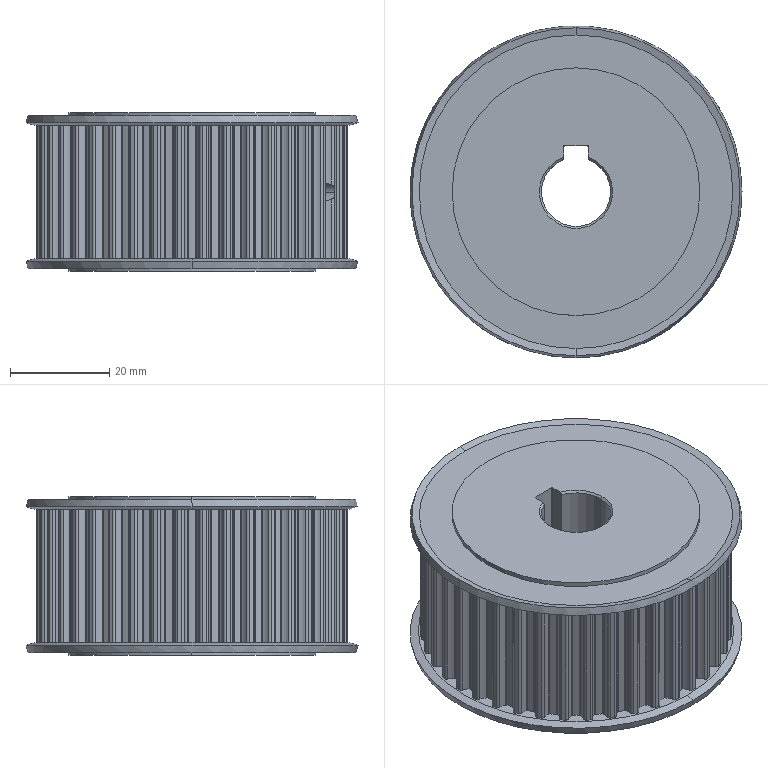Part | STEP file | EBJ52-S5M250-40-A-N-d14 | 1 solid | 408 faces | box 67 x 67 x 32 mm | volume 87087 mm3 | cylinder 381 | cone 18 | plane 9 | commonest cylinder face diameters 1.1 x99 0.5 x96 6.55 x90 59.16 x43 62.7 x40 4.134 x4